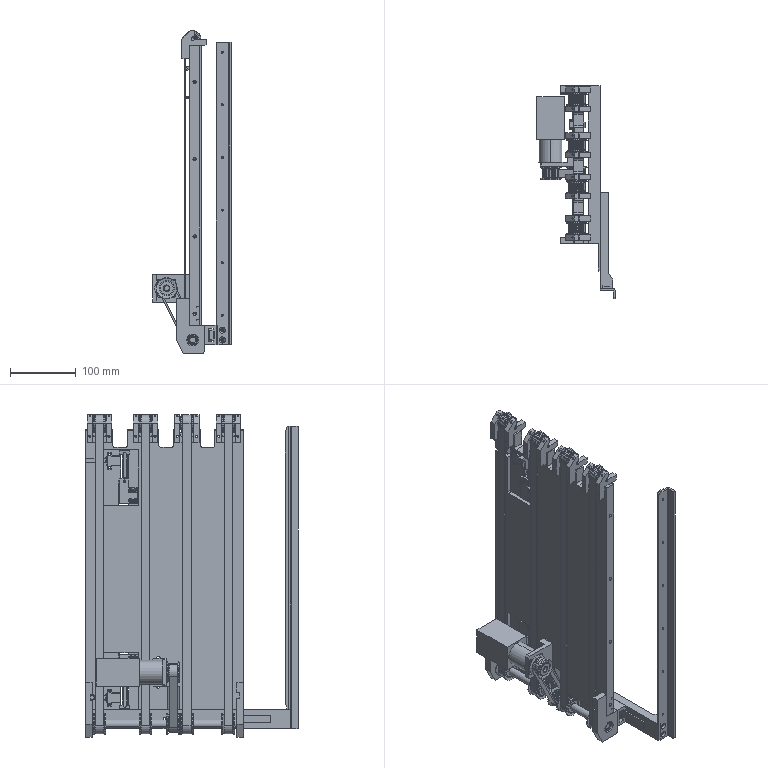Part | NX | features BREP 37 | 84 solids | 4815 faces | volume 2095053 mm3 | cylinder 2131 | plane 1816 | cone 452 | torus 232 | sphere 176 | spline 8 | commonest cylinder face diameters 1.22 x760 20.95 x170 23.75 x150 2.5 x116 4 x87 3.4 x84